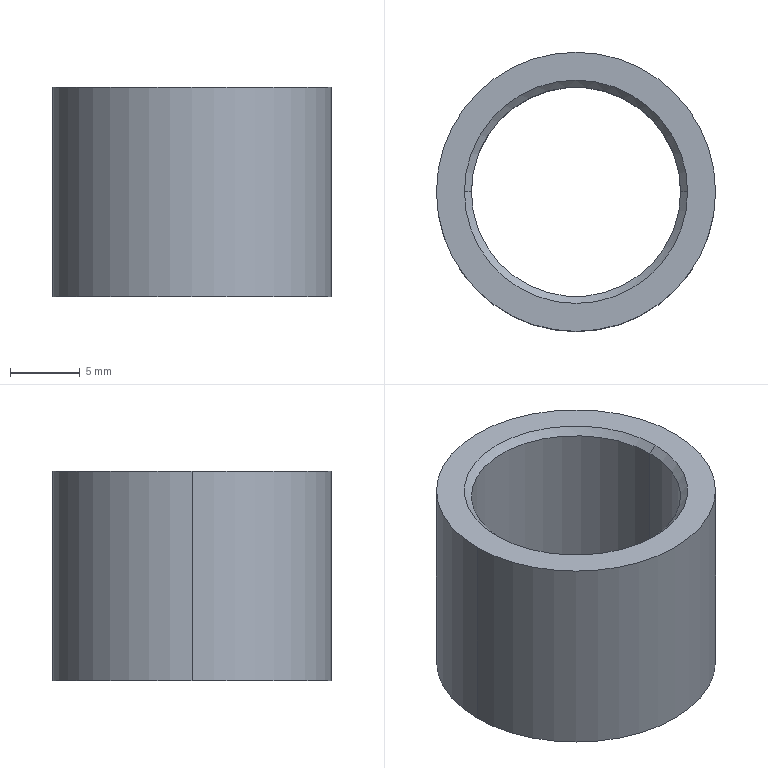Part | SolidWorks | features BaseBody 1 | 1 solid | 10 faces | box 20 x 20 x 15 mm | volume 2050 mm3 | cylinder 4 | cone 4 | plane 2 | commonest cylinder face diameters 15 x2 20 x2
STEP:
#1=CARTESIAN_POINT('',(-137.496,1831.544,-6.5));
#2=VERTEX_POINT('',#1);
#3=CARTESIAN_POINT('',(-117.496,1831.544,-6.5));
#4=VERTEX_POINT('',#3);
#5=CARTESIAN_POINT('',(-127.496,1831.544,-6.5));
#6=DIRECTION('',(0.,0.,-1.));
#7=DIRECTION('',(-1.,0.,0.));
#8=AXIS2_PLACEMENT_3D('',#5,#6,#7);
#9=CIRCLE('',#8,10.);
#10=EDGE_CURVE('',#2,#4,#9,.T.);
#11=ORIENTED_EDGE('',*,*,#10,.T.);
#12=CARTESIAN_POINT('',(-117.496,1831.544,-21.5));
#13=VERTEX_POINT('',#12);
#14=CARTESIAN_POINT('',(-117.496,1831.544,-21.5));
#15=DIRECTION('',(0.,0.,-1.));
#16=VECTOR('',#15,1000.);
#17=LINE('',#14,#16);
#18=EDGE_CURVE('',#4,#13,#17,.T.);
#19=ORIENTED_EDGE('',*,*,#18,.T.);
#20=CARTESIAN_POINT('',(-137.496,1831.544,-21.5));
#21=VERTEX_POINT('',#20);
#22=CARTESIAN_POINT('',(-127.496,1831.544,-21.5));
#23=DIRECTION('',(0.,0.,1.));
#24=DIRECTION('',(-1.,0.,0.));
#25=AXIS2_PLACEMENT_3D('',#22,#23,#24);
#26=CIRCLE('',#25,10.);
#27=EDGE_CURVE('',#13,#21,#26,.T.);
#28=ORIENTED_EDGE('',*,*,#27,.T.);
#29=CARTESIAN_POINT('',(-137.496,1831.544,-21.5));
#30=DIRECTION('',(0.,0.,-1.));
#31=VECTOR('',#30,1000.);
#32=LINE('',#29,#31);
#33=EDGE_CURVE('',#2,#21,#32,.T.);
#34=ORIENTED_EDGE('',*,*,#33,.F.);
#35=EDGE_LOOP('',(#11,#19,#28,#34));
#36=FACE_OUTER_BOUND('',#35,.T.);
#37=CARTESIAN_POINT('',(-127.496,1831.544,-21.5));
#38=DIRECTION('',(0.,0.,-1.));
#39=DIRECTION('',(-1.,0.,0.));
#40=AXIS2_PLACEMENT_3D('',#37,#38,#39);
#41=CYLINDRICAL_SURFACE('',#40,10.);
#42=ADVANCED_FACE('',(#36),#41,.T.);
#43=CARTESIAN_POINT('',(-119.996,1831.544,-21.));
#44=VERTEX_POINT('',#43);
#45=CARTESIAN_POINT('',(-134.996,1831.544,-21.));
#46=VERTEX_POINT('',#45);
#47=CARTESIAN_POINT('',(-127.496,1831.544,-21.));
#48=DIRECTION('',(0.,0.,-1.));
#49=DIRECTION('',(0.,-1.,0.));
#50=AXIS2_PLACEMENT_3D('',#47,#48,#49);
#51=CIRCLE('',#50,7.5);
#52=EDGE_CURVE('',#44,#46,#51,.T.);
#53=ORIENTED_EDGE('',*,*,#52,.F.);
#54=CARTESIAN_POINT('',(-119.496,1831.544,-21.5));
#55=VERTEX_POINT('',#54);
#56=CARTESIAN_POINT('',(-119.496,1831.544,-21.5));
#57=DIRECTION('',(0.7071,0.,-0.7071));
#58=VECTOR('',#57,1000.);
#59=LINE('',#56,#58);
#60=EDGE_CURVE('',#44,#55,#59,.T.);
#61=ORIENTED_EDGE('',*,*,#60,.T.);
#62=CARTESIAN_POINT('',(-135.496,1831.544,-21.5));
#63=VERTEX_POINT('',#62);
#64=CARTESIAN_POINT('',(-127.496,1831.544,-21.5));
#65=DIRECTION('',(0.,0.,-1.));
#66=DIRECTION('',(-1.,0.,0.));
#67=AXIS2_PLACEMENT_3D('',#64,#65,#66);
#68=CIRCLE('',#67,8.);
#69=EDGE_CURVE('',#55,#63,#68,.T.);
#70=ORIENTED_EDGE('',*,*,#69,.T.);
#71=CARTESIAN_POINT('',(-135.496,1831.544,-21.5));
#72=DIRECTION('',(-0.7071,0.,-0.7071));
#73=VECTOR('',#72,1000.);
#74=LINE('',#71,#73);
#75=EDGE_CURVE('',#46,#63,#74,.T.);
#76=ORIENTED_EDGE('',*,*,#75,.F.);
#77=EDGE_LOOP('',(#53,#61,#70,#76));
#78=FACE_OUTER_BOUND('',#77,.T.);
#79=CARTESIAN_POINT('',(-127.496,1831.544,-21.5));
#80=DIRECTION('',(0.,0.,-1.));
#81=DIRECTION('',(-1.,0.,0.));
#82=AXIS2_PLACEMENT_3D('',#79,#80,#81);
#83=CONICAL_SURFACE('',#82,8.,0.7854);
#84=ADVANCED_FACE('',(#78),#83,.F.);
#85=CARTESIAN_POINT('',(-134.996,1831.544,-7.));
#86=VERTEX_POINT('',#85);
#87=CARTESIAN_POINT('',(-119.996,1831.544,-7.));
#88=VERTEX_POINT('',#87);
#89=CARTESIAN_POINT('',(-127.496,1831.544,-7.));
#90=DIRECTION('',(0.,0.,1.));
#91=DIRECTION('',(0.,1.,0.));
#92=AXIS2_PLACEMENT_3D('',#89,#90,#91);
#93=CIRCLE('',#92,7.5);
#94=EDGE_CURVE('',#86,#88,#93,.T.);
#95=ORIENTED_EDGE('',*,*,#94,.F.);
#96=CARTESIAN_POINT('',(-135.496,1831.544,-6.5));
#97=VERTEX_POINT('',#96);
#98=CARTESIAN_POINT('',(-135.496,1831.544,-6.5));
#99=DIRECTION('',(-0.7071,0.,0.7071));
#100=VECTOR('',#99,1000.);
#101=LINE('',#98,#100);
#102=EDGE_CURVE('',#86,#97,#101,.T.);
#103=ORIENTED_EDGE('',*,*,#102,.T.);
#104=CARTESIAN_POINT('',(-119.496,1831.544,-6.5));
#105=VERTEX_POINT('',#104);
#106=CARTESIAN_POINT('',(-127.496,1831.544,-6.5));
#107=DIRECTION('',(0.,0.,1.));
#108=DIRECTION('',(1.,0.,0.));
#109=AXIS2_PLACEMENT_3D('',#106,#107,#108);
#110=CIRCLE('',#109,8.);
#111=EDGE_CURVE('',#97,#105,#110,.T.);
#112=ORIENTED_EDGE('',*,*,#111,.T.);
#113=CARTESIAN_POINT('',(-119.496,1831.544,-6.5));
#114=DIRECTION('',(0.7071,0.,0.7071));
#115=VECTOR('',#114,1000.);
#116=LINE('',#113,#115);
#117=EDGE_CURVE('',#88,#105,#116,.T.);
#118=ORIENTED_EDGE('',*,*,#117,.F.);
#119=EDGE_LOOP('',(#95,#103,#112,#118));
#120=FACE_OUTER_BOUND('',#119,.T.);
#121=CARTESIAN_POINT('',(-127.496,1831.544,-6.5));
#122=DIRECTION('',(0.,0.,1.));
#123=DIRECTION('',(1.,0.,0.));
#124=AXIS2_PLACEMENT_3D('',#121,#122,#123);
#125=CONICAL_SURFACE('',#124,8.,0.7854);
#126=ADVANCED_FACE('',(#120),#125,.F.);
#127=ORIENTED_EDGE('',*,*,#94,.T.);
#128=CARTESIAN_POINT('',(-119.996,1831.544,-21.5));
#129=DIRECTION('',(0.,0.,-1.));
#130=VECTOR('',#129,1000.);
#131=LINE('',#128,#130);
#132=EDGE_CURVE('',#88,#44,#131,.T.);
#133=ORIENTED_EDGE('',*,*,#132,.T.);
#134=ORIENTED_EDGE('',*,*,#52,.T.);
#135=CARTESIAN_POINT('',(-134.996,1831.544,-21.5));
#136=DIRECTION('',(0.,0.,-1.));
#137=VECTOR('',#136,1000.);
#138=LINE('',#135,#137);
#139=EDGE_CURVE('',#86,#46,#138,.T.);
#140=ORIENTED_EDGE('',*,*,#139,.F.);
#141=EDGE_LOOP('',(#127,#133,#134,#140));
#142=FACE_OUTER_BOUND('',#141,.T.);
#143=CARTESIAN_POINT('',(-127.496,1831.544,-21.5));
#144=DIRECTION('',(0.,0.,-1.));
#145=DIRECTION('',(-1.,0.,0.));
#146=AXIS2_PLACEMENT_3D('',#143,#144,#145);
#147=CYLINDRICAL_SURFACE('',#146,7.5);
#148=ADVANCED_FACE('',(#142),#147,.F.);
#149=ORIENTED_EDGE('',*,*,#18,.F.);
#150=CARTESIAN_POINT('',(-127.496,1831.544,-6.5));
#151=DIRECTION('',(0.,0.,-1.));
#152=DIRECTION('',(-1.,0.,0.));
#153=AXIS2_PLACEMENT_3D('',#150,#151,#152);
#154=CIRCLE('',#153,10.);
#155=EDGE_CURVE('',#4,#2,#154,.T.);
#156=ORIENTED_EDGE('',*,*,#155,.T.);
#157=ORIENTED_EDGE('',*,*,#33,.T.);
#158=CARTESIAN_POINT('',(-127.496,1831.544,-21.5));
#159=DIRECTION('',(0.,0.,1.));
#160=DIRECTION('',(-1.,0.,0.));
#161=AXIS2_PLACEMENT_3D('',#158,#159,#160);
#162=CIRCLE('',#161,10.);
#163=EDGE_CURVE('',#21,#13,#162,.T.);
#164=ORIENTED_EDGE('',*,*,#163,.T.);
#165=EDGE_LOOP('',(#149,#156,#157,#164));
#166=FACE_OUTER_BOUND('',#165,.T.);
#167=CARTESIAN_POINT('',(-127.496,1831.544,-21.5));
#168=DIRECTION('',(0.,0.,-1.));
#169=DIRECTION('',(-1.,0.,0.));
#170=AXIS2_PLACEMENT_3D('',#167,#168,#169);
#171=CYLINDRICAL_SURFACE('',#170,10.);
#172=ADVANCED_FACE('',(#166),#171,.T.);
#173=CARTESIAN_POINT('',(-127.496,1831.544,-21.5));
#174=DIRECTION('',(0.,0.,-1.));
#175=DIRECTION('',(-1.,0.,0.));
#176=AXIS2_PLACEMENT_3D('',#173,#174,#175);
#177=CIRCLE('',#176,8.);
#178=EDGE_CURVE('',#63,#55,#177,.T.);
#179=ORIENTED_EDGE('',*,*,#178,.F.);
#180=ORIENTED_EDGE('',*,*,#69,.F.);
#181=EDGE_LOOP('',(#179,#180));
#182=FACE_BOUND('',#181,.T.);
#183=ORIENTED_EDGE('',*,*,#163,.F.);
#184=ORIENTED_EDGE('',*,*,#27,.F.);
#185=EDGE_LOOP('',(#183,#184));
#186=FACE_OUTER_BOUND('',#185,.T.);
#187=CARTESIAN_POINT('',(-137.496,1831.544,-21.5));
#188=DIRECTION('',(0.,0.,1.));
#189=DIRECTION('',(1.,0.,0.));
#190=AXIS2_PLACEMENT_3D('',#187,#188,#189);
#191=PLANE('',#190);
#192=ADVANCED_FACE('',(#182,#186),#191,.F.);
#193=CARTESIAN_POINT('',(-127.496,1831.544,-6.5));
#194=DIRECTION('',(0.,0.,1.));
#195=DIRECTION('',(1.,0.,0.));
#196=AXIS2_PLACEMENT_3D('',#193,#194,#195);
#197=CIRCLE('',#196,8.);
#198=EDGE_CURVE('',#105,#97,#197,.T.);
#199=ORIENTED_EDGE('',*,*,#198,.F.);
#200=ORIENTED_EDGE('',*,*,#111,.F.);
#201=EDGE_LOOP('',(#199,#200));
#202=FACE_BOUND('',#201,.T.);
#203=ORIENTED_EDGE('',*,*,#10,.F.);
#204=ORIENTED_EDGE('',*,*,#155,.F.);
#205=EDGE_LOOP('',(#203,#204));
#206=FACE_OUTER_BOUND('',#205,.T.);
#207=CARTESIAN_POINT('',(-134.996,1831.544,-6.5));
#208=DIRECTION('',(0.,0.,-1.));
#209=DIRECTION('',(-1.,0.,0.));
#210=AXIS2_PLACEMENT_3D('',#207,#208,#209);
#211=PLANE('',#210);
#212=ADVANCED_FACE('',(#202,#206),#211,.F.);
#213=ORIENTED_EDGE('',*,*,#60,.F.);
#214=CARTESIAN_POINT('',(-127.496,1831.544,-21.));
#215=DIRECTION('',(0.,0.,-1.));
#216=DIRECTION('',(0.,-1.,0.));
#217=AXIS2_PLACEMENT_3D('',#214,#215,#216);
#218=CIRCLE('',#217,7.5);
#219=EDGE_CURVE('',#46,#44,#218,.T.);
#220=ORIENTED_EDGE('',*,*,#219,.F.);
#221=ORIENTED_EDGE('',*,*,#75,.T.);
#222=ORIENTED_EDGE('',*,*,#178,.T.);
#223=EDGE_LOOP('',(#213,#220,#221,#222));
#224=FACE_OUTER_BOUND('',#223,.T.);
#225=CARTESIAN_POINT('',(-127.496,1831.544,-21.5));
#226=DIRECTION('',(0.,0.,-1.));
#227=DIRECTION('',(-1.,0.,0.));
#228=AXIS2_PLACEMENT_3D('',#225,#226,#227);
#229=CONICAL_SURFACE('',#228,8.,0.7854);
#230=ADVANCED_FACE('',(#224),#229,.F.);
#231=ORIENTED_EDGE('',*,*,#102,.F.);
#232=CARTESIAN_POINT('',(-127.496,1831.544,-7.));
#233=DIRECTION('',(0.,0.,1.));
#234=DIRECTION('',(0.,1.,0.));
#235=AXIS2_PLACEMENT_3D('',#232,#233,#234);
#236=CIRCLE('',#235,7.5);
#237=EDGE_CURVE('',#88,#86,#236,.T.);
#238=ORIENTED_EDGE('',*,*,#237,.F.);
#239=ORIENTED_EDGE('',*,*,#117,.T.);
#240=ORIENTED_EDGE('',*,*,#198,.T.);
#241=EDGE_LOOP('',(#231,#238,#239,#240));
#242=FACE_OUTER_BOUND('',#241,.T.);
#243=CARTESIAN_POINT('',(-127.496,1831.544,-6.5));
#244=DIRECTION('',(0.,0.,1.));
#245=DIRECTION('',(1.,0.,0.));
#246=AXIS2_PLACEMENT_3D('',#243,#244,#245);
#247=CONICAL_SURFACE('',#246,8.,0.7854);
#248=ADVANCED_FACE('',(#242),#247,.F.);
#249=ORIENTED_EDGE('',*,*,#132,.F.);
#250=ORIENTED_EDGE('',*,*,#237,.T.);
#251=ORIENTED_EDGE('',*,*,#139,.T.);
#252=ORIENTED_EDGE('',*,*,#219,.T.);
#253=EDGE_LOOP('',(#249,#250,#251,#252));
#254=FACE_OUTER_BOUND('',#253,.T.);
#255=CARTESIAN_POINT('',(-127.496,1831.544,-21.5));
#256=DIRECTION('',(0.,0.,-1.));
#257=DIRECTION('',(-1.,0.,0.));
#258=AXIS2_PLACEMENT_3D('',#255,#256,#257);
#259=CYLINDRICAL_SURFACE('',#258,7.5);
#260=ADVANCED_FACE('',(#254),#259,.F.);
#261=CLOSED_SHELL('',(#42,#84,#126,#148,#172,#192,#212,#230,#248,#260));
#262=MANIFOLD_SOLID_BREP('',#261);
#263=CARTESIAN_POINT('',(0.,0.,0.));
#264=DIRECTION('',(0.,0.,1.));
#265=DIRECTION('',(1.,0.,0.));
#266=AXIS2_PLACEMENT_3D('',#263,#264,#265);
#267=(LENGTH_UNIT()NAMED_UNIT(*)SI_UNIT(.MILLI.,.METRE.));
#268=UNCERTAINTY_MEASURE_WITH_UNIT(LENGTH_MEASURE(0.00001),#267,'','');
#269=(NAMED_UNIT(*)PLANE_ANGLE_UNIT()SI_UNIT($,.RADIAN.));
#270=(NAMED_UNIT(*)SI_UNIT($,.STERADIAN.)SOLID_ANGLE_UNIT());
#271=(GEOMETRIC_REPRESENTATION_CONTEXT(3)GLOBAL_UNCERTAINTY_ASSIGNED_CONTEXT((#268))GLOBAL_UNIT_ASSIGNED_CONTEXT((#267,#269,#270))REPRESENTATION_CONTEXT('',''));
#272=ADVANCED_BREP_SHAPE_REPRESENTATION('',(#262,#266),#271);